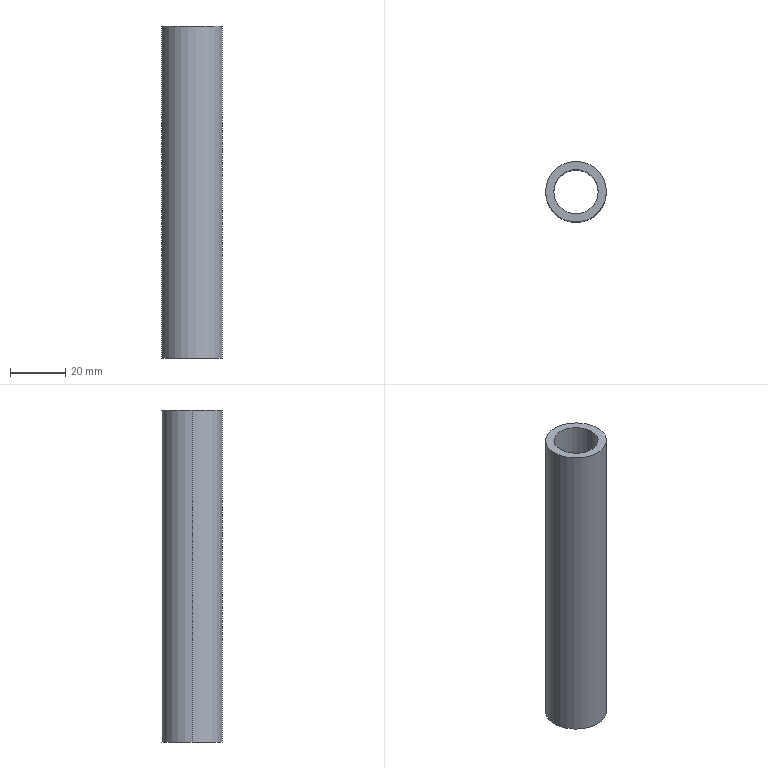Part | SolidWorks | features Extrusion 1 | 1 solid | 6 faces | box 22 x 22 x 120 mm | volume 21488 mm3 | cylinder 4 | plane 2 | commonest cylinder face diameters 16 x2 22 x2
STEP:
#1=CARTESIAN_POINT('',(-8.,0.,120.));
#2=VERTEX_POINT('',#1);
#3=CARTESIAN_POINT('',(8.,0.,120.));
#4=VERTEX_POINT('',#3);
#5=CARTESIAN_POINT('',(0.,0.,120.));
#6=DIRECTION('',(0.,0.,1.));
#7=DIRECTION('',(1.,0.,0.));
#8=AXIS2_PLACEMENT_3D('',#5,#6,#7);
#9=CIRCLE('',#8,8.);
#10=EDGE_CURVE('',#2,#4,#9,.T.);
#11=ORIENTED_EDGE('',*,*,#10,.T.);
#12=CARTESIAN_POINT('',(8.,0.,0.));
#13=VERTEX_POINT('',#12);
#14=CARTESIAN_POINT('',(8.,0.,120.));
#15=DIRECTION('',(0.,0.,-1.));
#16=VECTOR('',#15,1000.);
#17=LINE('',#14,#16);
#18=EDGE_CURVE('',#4,#13,#17,.T.);
#19=ORIENTED_EDGE('',*,*,#18,.T.);
#20=CARTESIAN_POINT('',(-8.,0.,0.));
#21=VERTEX_POINT('',#20);
#22=CARTESIAN_POINT('',(0.,0.,0.));
#23=DIRECTION('',(0.,0.,1.));
#24=DIRECTION('',(1.,0.,0.));
#25=AXIS2_PLACEMENT_3D('',#22,#23,#24);
#26=CIRCLE('',#25,8.);
#27=EDGE_CURVE('',#21,#13,#26,.T.);
#28=ORIENTED_EDGE('',*,*,#27,.F.);
#29=CARTESIAN_POINT('',(-8.,0.,120.));
#30=DIRECTION('',(0.,0.,-1.));
#31=VECTOR('',#30,1000.);
#32=LINE('',#29,#31);
#33=EDGE_CURVE('',#2,#21,#32,.T.);
#34=ORIENTED_EDGE('',*,*,#33,.F.);
#35=EDGE_LOOP('',(#11,#19,#28,#34));
#36=FACE_OUTER_BOUND('',#35,.T.);
#37=CARTESIAN_POINT('',(0.,0.,120.));
#38=DIRECTION('',(0.,0.,-1.));
#39=DIRECTION('',(-1.,0.,0.));
#40=AXIS2_PLACEMENT_3D('',#37,#38,#39);
#41=CYLINDRICAL_SURFACE('',#40,8.);
#42=ADVANCED_FACE('',(#36),#41,.F.);
#43=CARTESIAN_POINT('',(11.,0.,120.));
#44=VERTEX_POINT('',#43);
#45=CARTESIAN_POINT('',(-11.,0.,120.));
#46=VERTEX_POINT('',#45);
#47=CARTESIAN_POINT('',(0.,0.,120.));
#48=DIRECTION('',(0.,0.,1.));
#49=DIRECTION('',(1.,0.,0.));
#50=AXIS2_PLACEMENT_3D('',#47,#48,#49);
#51=CIRCLE('',#50,11.);
#52=EDGE_CURVE('',#44,#46,#51,.T.);
#53=ORIENTED_EDGE('',*,*,#52,.F.);
#54=CARTESIAN_POINT('',(11.,0.,0.));
#55=VERTEX_POINT('',#54);
#56=CARTESIAN_POINT('',(11.,0.,120.));
#57=DIRECTION('',(0.,0.,-1.));
#58=VECTOR('',#57,1000.);
#59=LINE('',#56,#58);
#60=EDGE_CURVE('',#44,#55,#59,.T.);
#61=ORIENTED_EDGE('',*,*,#60,.T.);
#62=CARTESIAN_POINT('',(-11.,0.,0.));
#63=VERTEX_POINT('',#62);
#64=CARTESIAN_POINT('',(0.,0.,0.));
#65=DIRECTION('',(0.,0.,1.));
#66=DIRECTION('',(1.,0.,0.));
#67=AXIS2_PLACEMENT_3D('',#64,#65,#66);
#68=CIRCLE('',#67,11.);
#69=EDGE_CURVE('',#55,#63,#68,.T.);
#70=ORIENTED_EDGE('',*,*,#69,.T.);
#71=CARTESIAN_POINT('',(-11.,0.,120.));
#72=DIRECTION('',(0.,0.,-1.));
#73=VECTOR('',#72,1000.);
#74=LINE('',#71,#73);
#75=EDGE_CURVE('',#46,#63,#74,.T.);
#76=ORIENTED_EDGE('',*,*,#75,.F.);
#77=EDGE_LOOP('',(#53,#61,#70,#76));
#78=FACE_OUTER_BOUND('',#77,.T.);
#79=CARTESIAN_POINT('',(0.,0.,120.));
#80=DIRECTION('',(0.,0.,-1.));
#81=DIRECTION('',(-1.,0.,0.));
#82=AXIS2_PLACEMENT_3D('',#79,#80,#81);
#83=CYLINDRICAL_SURFACE('',#82,11.);
#84=ADVANCED_FACE('',(#78),#83,.T.);
#85=CARTESIAN_POINT('',(0.,0.,120.));
#86=DIRECTION('',(0.,0.,1.));
#87=DIRECTION('',(1.,0.,0.));
#88=AXIS2_PLACEMENT_3D('',#85,#86,#87);
#89=CIRCLE('',#88,11.);
#90=EDGE_CURVE('',#46,#44,#89,.T.);
#91=ORIENTED_EDGE('',*,*,#90,.T.);
#92=ORIENTED_EDGE('',*,*,#52,.T.);
#93=EDGE_LOOP('',(#91,#92));
#94=FACE_OUTER_BOUND('',#93,.T.);
#95=ORIENTED_EDGE('',*,*,#10,.F.);
#96=CARTESIAN_POINT('',(0.,0.,120.));
#97=DIRECTION('',(0.,0.,1.));
#98=DIRECTION('',(1.,0.,0.));
#99=AXIS2_PLACEMENT_3D('',#96,#97,#98);
#100=CIRCLE('',#99,8.);
#101=EDGE_CURVE('',#4,#2,#100,.T.);
#102=ORIENTED_EDGE('',*,*,#101,.F.);
#103=EDGE_LOOP('',(#95,#102));
#104=FACE_BOUND('',#103,.T.);
#105=CARTESIAN_POINT('',(0.,0.,120.));
#106=DIRECTION('',(0.,0.,1.));
#107=DIRECTION('',(1.,0.,0.));
#108=AXIS2_PLACEMENT_3D('',#105,#106,#107);
#109=PLANE('',#108);
#110=ADVANCED_FACE('',(#94,#104),#109,.T.);
#111=CARTESIAN_POINT('',(0.,0.,0.));
#112=DIRECTION('',(0.,0.,1.));
#113=DIRECTION('',(1.,0.,0.));
#114=AXIS2_PLACEMENT_3D('',#111,#112,#113);
#115=CIRCLE('',#114,11.);
#116=EDGE_CURVE('',#63,#55,#115,.T.);
#117=ORIENTED_EDGE('',*,*,#116,.F.);
#118=ORIENTED_EDGE('',*,*,#69,.F.);
#119=EDGE_LOOP('',(#117,#118));
#120=FACE_OUTER_BOUND('',#119,.T.);
#121=ORIENTED_EDGE('',*,*,#27,.T.);
#122=CARTESIAN_POINT('',(0.,0.,0.));
#123=DIRECTION('',(0.,0.,1.));
#124=DIRECTION('',(1.,0.,0.));
#125=AXIS2_PLACEMENT_3D('',#122,#123,#124);
#126=CIRCLE('',#125,8.);
#127=EDGE_CURVE('',#13,#21,#126,.T.);
#128=ORIENTED_EDGE('',*,*,#127,.T.);
#129=EDGE_LOOP('',(#121,#128));
#130=FACE_BOUND('',#129,.T.);
#131=CARTESIAN_POINT('',(0.,0.,0.));
#132=DIRECTION('',(0.,0.,1.));
#133=DIRECTION('',(1.,0.,0.));
#134=AXIS2_PLACEMENT_3D('',#131,#132,#133);
#135=PLANE('',#134);
#136=ADVANCED_FACE('',(#120,#130),#135,.F.);
#137=ORIENTED_EDGE('',*,*,#60,.F.);
#138=ORIENTED_EDGE('',*,*,#90,.F.);
#139=ORIENTED_EDGE('',*,*,#75,.T.);
#140=ORIENTED_EDGE('',*,*,#116,.T.);
#141=EDGE_LOOP('',(#137,#138,#139,#140));
#142=FACE_OUTER_BOUND('',#141,.T.);
#143=CARTESIAN_POINT('',(0.,0.,120.));
#144=DIRECTION('',(0.,0.,-1.));
#145=DIRECTION('',(-1.,0.,0.));
#146=AXIS2_PLACEMENT_3D('',#143,#144,#145);
#147=CYLINDRICAL_SURFACE('',#146,11.);
#148=ADVANCED_FACE('',(#142),#147,.T.);
#149=ORIENTED_EDGE('',*,*,#18,.F.);
#150=ORIENTED_EDGE('',*,*,#101,.T.);
#151=ORIENTED_EDGE('',*,*,#33,.T.);
#152=ORIENTED_EDGE('',*,*,#127,.F.);
#153=EDGE_LOOP('',(#149,#150,#151,#152));
#154=FACE_OUTER_BOUND('',#153,.T.);
#155=CARTESIAN_POINT('',(0.,0.,120.));
#156=DIRECTION('',(0.,0.,-1.));
#157=DIRECTION('',(-1.,0.,0.));
#158=AXIS2_PLACEMENT_3D('',#155,#156,#157);
#159=CYLINDRICAL_SURFACE('',#158,8.);
#160=ADVANCED_FACE('',(#154),#159,.F.);
#161=CLOSED_SHELL('',(#42,#84,#110,#136,#148,#160));
#162=MANIFOLD_SOLID_BREP('',#161);
#163=CARTESIAN_POINT('',(0.,0.,0.));
#164=DIRECTION('',(0.,0.,1.));
#165=DIRECTION('',(1.,0.,0.));
#166=AXIS2_PLACEMENT_3D('',#163,#164,#165);
#167=(LENGTH_UNIT()NAMED_UNIT(*)SI_UNIT(.MILLI.,.METRE.));
#168=UNCERTAINTY_MEASURE_WITH_UNIT(LENGTH_MEASURE(0.00001),#167,'','');
#169=(NAMED_UNIT(*)PLANE_ANGLE_UNIT()SI_UNIT($,.RADIAN.));
#170=(NAMED_UNIT(*)SI_UNIT($,.STERADIAN.)SOLID_ANGLE_UNIT());
#171=(GEOMETRIC_REPRESENTATION_CONTEXT(3)GLOBAL_UNCERTAINTY_ASSIGNED_CONTEXT((#168))GLOBAL_UNIT_ASSIGNED_CONTEXT((#167,#169,#170))REPRESENTATION_CONTEXT('',''));
#172=ADVANCED_BREP_SHAPE_REPRESENTATION('',(#162,#166),#171);